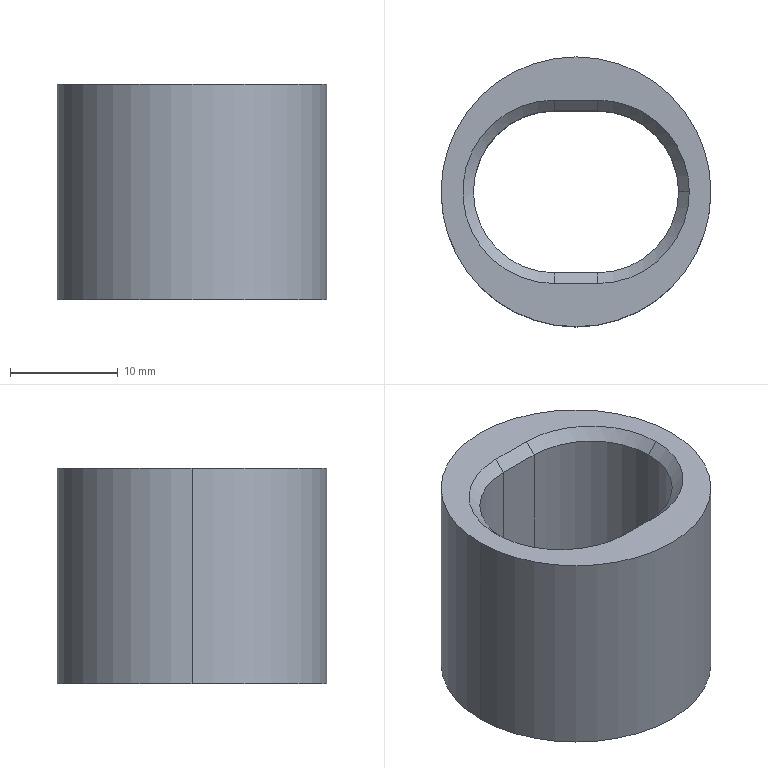Part | SolidWorks | features Chamfer 1, Extrusion 1 | 1 solid | 14 faces | box 25 x 25 x 20 mm | volume 5055 mm3 | plane 6 | cylinder 5 | cone 3 | commonest cylinder face diameters 15 x3 25 x2
STEP:
#1=CARTESIAN_POINT('',(9.5,0.,19.));
#2=VERTEX_POINT('',#1);
#3=CARTESIAN_POINT('',(2.,7.5,19.));
#4=VERTEX_POINT('',#3);
#5=CARTESIAN_POINT('',(2.,0.,19.));
#6=DIRECTION('',(0.,0.,1.));
#7=DIRECTION('',(1.,0.,0.));
#8=AXIS2_PLACEMENT_3D('',#5,#6,#7);
#9=CIRCLE('',#8,7.5);
#10=EDGE_CURVE('',#2,#4,#9,.T.);
#11=ORIENTED_EDGE('',*,*,#10,.F.);
#12=CARTESIAN_POINT('',(10.5,0.,20.));
#13=VERTEX_POINT('',#12);
#14=CARTESIAN_POINT('',(9.5,0.,19.));
#15=DIRECTION('',(0.7071,0.,0.7071));
#16=VECTOR('',#15,1000.);
#17=LINE('',#14,#16);
#18=EDGE_CURVE('',#2,#13,#17,.T.);
#19=ORIENTED_EDGE('',*,*,#18,.T.);
#20=CARTESIAN_POINT('',(2.,8.5,20.));
#21=VERTEX_POINT('',#20);
#22=CARTESIAN_POINT('',(2.,0.,20.));
#23=DIRECTION('',(0.,0.,-1.));
#24=DIRECTION('',(1.,0.,0.));
#25=AXIS2_PLACEMENT_3D('',#22,#23,#24);
#26=CIRCLE('',#25,8.5);
#27=EDGE_CURVE('',#21,#13,#26,.T.);
#28=ORIENTED_EDGE('',*,*,#27,.F.);
#29=CARTESIAN_POINT('',(2.,8.5,20.));
#30=DIRECTION('',(0.,-0.7071,-0.7071));
#31=VECTOR('',#30,1000.);
#32=LINE('',#29,#31);
#33=EDGE_CURVE('',#21,#4,#32,.T.);
#34=ORIENTED_EDGE('',*,*,#33,.T.);
#35=EDGE_LOOP('',(#11,#19,#28,#34));
#36=FACE_OUTER_BOUND('',#35,.T.);
#37=CARTESIAN_POINT('',(2.,0.,19.));
#38=DIRECTION('',(0.,0.,1.));
#39=DIRECTION('',(1.,0.,0.));
#40=AXIS2_PLACEMENT_3D('',#37,#38,#39);
#41=CONICAL_SURFACE('',#40,7.5,0.7854);
#42=ADVANCED_FACE('',(#36),#41,.F.);
#43=CARTESIAN_POINT('',(-2.,7.5,19.));
#44=VERTEX_POINT('',#43);
#45=CARTESIAN_POINT('',(-9.5,0.,19.));
#46=VERTEX_POINT('',#45);
#47=CARTESIAN_POINT('',(-2.,0.,19.));
#48=DIRECTION('',(0.,0.,1.));
#49=DIRECTION('',(1.,0.,0.));
#50=AXIS2_PLACEMENT_3D('',#47,#48,#49);
#51=CIRCLE('',#50,7.5);
#52=EDGE_CURVE('',#44,#46,#51,.T.);
#53=ORIENTED_EDGE('',*,*,#52,.T.);
#54=CARTESIAN_POINT('',(-9.5,0.,0.));
#55=VERTEX_POINT('',#54);
#56=CARTESIAN_POINT('',(-9.5,0.,20.));
#57=DIRECTION('',(0.,0.,-1.));
#58=VECTOR('',#57,1000.);
#59=LINE('',#56,#58);
#60=EDGE_CURVE('',#46,#55,#59,.T.);
#61=ORIENTED_EDGE('',*,*,#60,.T.);
#62=CARTESIAN_POINT('',(-2.,7.5,0.));
#63=VERTEX_POINT('',#62);
#64=CARTESIAN_POINT('',(-2.,0.,0.));
#65=DIRECTION('',(0.,0.,1.));
#66=DIRECTION('',(1.,0.,0.));
#67=AXIS2_PLACEMENT_3D('',#64,#65,#66);
#68=CIRCLE('',#67,7.5);
#69=EDGE_CURVE('',#63,#55,#68,.T.);
#70=ORIENTED_EDGE('',*,*,#69,.F.);
#71=CARTESIAN_POINT('',(-2.,7.5,20.));
#72=DIRECTION('',(0.,0.,-1.));
#73=VECTOR('',#72,1000.);
#74=LINE('',#71,#73);
#75=EDGE_CURVE('',#44,#63,#74,.T.);
#76=ORIENTED_EDGE('',*,*,#75,.F.);
#77=EDGE_LOOP('',(#53,#61,#70,#76));
#78=FACE_OUTER_BOUND('',#77,.T.);
#79=CARTESIAN_POINT('',(-2.,0.,20.));
#80=DIRECTION('',(0.,0.,-1.));
#81=DIRECTION('',(-1.,0.,0.));
#82=AXIS2_PLACEMENT_3D('',#79,#80,#81);
#83=CYLINDRICAL_SURFACE('',#82,7.5);
#84=ADVANCED_FACE('',(#78),#83,.F.);
#85=CARTESIAN_POINT('',(12.5,0.,20.));
#86=VERTEX_POINT('',#85);
#87=CARTESIAN_POINT('',(-12.5,0.,20.));
#88=VERTEX_POINT('',#87);
#89=CARTESIAN_POINT('',(0.,0.,20.));
#90=DIRECTION('',(0.,0.,1.));
#91=DIRECTION('',(1.,0.,0.));
#92=AXIS2_PLACEMENT_3D('',#89,#90,#91);
#93=CIRCLE('',#92,12.5);
#94=EDGE_CURVE('',#86,#88,#93,.T.);
#95=ORIENTED_EDGE('',*,*,#94,.F.);
#96=CARTESIAN_POINT('',(12.5,0.,0.));
#97=VERTEX_POINT('',#96);
#98=CARTESIAN_POINT('',(12.5,0.,20.));
#99=DIRECTION('',(0.,0.,-1.));
#100=VECTOR('',#99,1000.);
#101=LINE('',#98,#100);
#102=EDGE_CURVE('',#86,#97,#101,.T.);
#103=ORIENTED_EDGE('',*,*,#102,.T.);
#104=CARTESIAN_POINT('',(-12.5,0.,0.));
#105=VERTEX_POINT('',#104);
#106=CARTESIAN_POINT('',(0.,0.,0.));
#107=DIRECTION('',(0.,0.,1.));
#108=DIRECTION('',(1.,0.,0.));
#109=AXIS2_PLACEMENT_3D('',#106,#107,#108);
#110=CIRCLE('',#109,12.5);
#111=EDGE_CURVE('',#97,#105,#110,.T.);
#112=ORIENTED_EDGE('',*,*,#111,.T.);
#113=CARTESIAN_POINT('',(-12.5,0.,20.));
#114=DIRECTION('',(0.,0.,-1.));
#115=VECTOR('',#114,1000.);
#116=LINE('',#113,#115);
#117=EDGE_CURVE('',#88,#105,#116,.T.);
#118=ORIENTED_EDGE('',*,*,#117,.F.);
#119=EDGE_LOOP('',(#95,#103,#112,#118));
#120=FACE_OUTER_BOUND('',#119,.T.);
#121=CARTESIAN_POINT('',(0.,0.,20.));
#122=DIRECTION('',(0.,0.,-1.));
#123=DIRECTION('',(-1.,0.,0.));
#124=AXIS2_PLACEMENT_3D('',#121,#122,#123);
#125=CYLINDRICAL_SURFACE('',#124,12.5);
#126=ADVANCED_FACE('',(#120),#125,.T.);
#127=ORIENTED_EDGE('',*,*,#27,.T.);
#128=CARTESIAN_POINT('',(2.,-8.5,20.));
#129=VERTEX_POINT('',#128);
#130=CARTESIAN_POINT('',(2.,0.,20.));
#131=DIRECTION('',(0.,0.,-1.));
#132=DIRECTION('',(1.,0.,0.));
#133=AXIS2_PLACEMENT_3D('',#130,#131,#132);
#134=CIRCLE('',#133,8.5);
#135=EDGE_CURVE('',#13,#129,#134,.T.);
#136=ORIENTED_EDGE('',*,*,#135,.T.);
#137=CARTESIAN_POINT('',(-2.,-8.5,20.));
#138=VERTEX_POINT('',#137);
#139=CARTESIAN_POINT('',(0.,-8.5,20.));
#140=DIRECTION('',(-1.,0.,0.));
#141=VECTOR('',#140,1000.);
#142=LINE('',#139,#141);
#143=EDGE_CURVE('',#129,#138,#142,.T.);
#144=ORIENTED_EDGE('',*,*,#143,.T.);
#145=CARTESIAN_POINT('',(-2.,8.5,20.));
#146=VERTEX_POINT('',#145);
#147=CARTESIAN_POINT('',(-2.,0.,20.));
#148=DIRECTION('',(0.,0.,-1.));
#149=DIRECTION('',(1.,0.,0.));
#150=AXIS2_PLACEMENT_3D('',#147,#148,#149);
#151=CIRCLE('',#150,8.5);
#152=EDGE_CURVE('',#138,#146,#151,.T.);
#153=ORIENTED_EDGE('',*,*,#152,.T.);
#154=CARTESIAN_POINT('',(0.,8.5,20.));
#155=DIRECTION('',(1.,0.,0.));
#156=VECTOR('',#155,1000.);
#157=LINE('',#154,#156);
#158=EDGE_CURVE('',#146,#21,#157,.T.);
#159=ORIENTED_EDGE('',*,*,#158,.T.);
#160=EDGE_LOOP('',(#127,#136,#144,#153,#159));
#161=FACE_BOUND('',#160,.T.);
#162=CARTESIAN_POINT('',(0.,0.,20.));
#163=DIRECTION('',(0.,0.,1.));
#164=DIRECTION('',(1.,0.,0.));
#165=AXIS2_PLACEMENT_3D('',#162,#163,#164);
#166=CIRCLE('',#165,12.5);
#167=EDGE_CURVE('',#88,#86,#166,.T.);
#168=ORIENTED_EDGE('',*,*,#167,.T.);
#169=ORIENTED_EDGE('',*,*,#94,.T.);
#170=EDGE_LOOP('',(#168,#169));
#171=FACE_OUTER_BOUND('',#170,.T.);
#172=CARTESIAN_POINT('',(0.,0.,20.));
#173=DIRECTION('',(0.,0.,1.));
#174=DIRECTION('',(1.,0.,0.));
#175=AXIS2_PLACEMENT_3D('',#172,#173,#174);
#176=PLANE('',#175);
#177=ADVANCED_FACE('',(#161,#171),#176,.T.);
#178=CARTESIAN_POINT('',(0.,0.,0.));
#179=DIRECTION('',(0.,0.,1.));
#180=DIRECTION('',(1.,0.,0.));
#181=AXIS2_PLACEMENT_3D('',#178,#179,#180);
#182=CIRCLE('',#181,12.5);
#183=EDGE_CURVE('',#105,#97,#182,.T.);
#184=ORIENTED_EDGE('',*,*,#183,.F.);
#185=ORIENTED_EDGE('',*,*,#111,.F.);
#186=EDGE_LOOP('',(#184,#185));
#187=FACE_OUTER_BOUND('',#186,.T.);
#188=ORIENTED_EDGE('',*,*,#69,.T.);
#189=CARTESIAN_POINT('',(-2.,-7.5,0.));
#190=VERTEX_POINT('',#189);
#191=CARTESIAN_POINT('',(-2.,0.,0.));
#192=DIRECTION('',(0.,0.,1.));
#193=DIRECTION('',(1.,0.,0.));
#194=AXIS2_PLACEMENT_3D('',#191,#192,#193);
#195=CIRCLE('',#194,7.5);
#196=EDGE_CURVE('',#55,#190,#195,.T.);
#197=ORIENTED_EDGE('',*,*,#196,.T.);
#198=CARTESIAN_POINT('',(2.,-7.5,0.));
#199=VERTEX_POINT('',#198);
#200=CARTESIAN_POINT('',(-2.,-7.5,0.));
#201=DIRECTION('',(1.,0.,0.));
#202=VECTOR('',#201,1000.);
#203=LINE('',#200,#202);
#204=EDGE_CURVE('',#190,#199,#203,.T.);
#205=ORIENTED_EDGE('',*,*,#204,.T.);
#206=CARTESIAN_POINT('',(2.,7.5,0.));
#207=VERTEX_POINT('',#206);
#208=CARTESIAN_POINT('',(2.,0.,0.));
#209=DIRECTION('',(0.,0.,1.));
#210=DIRECTION('',(1.,0.,0.));
#211=AXIS2_PLACEMENT_3D('',#208,#209,#210);
#212=CIRCLE('',#211,7.5);
#213=EDGE_CURVE('',#199,#207,#212,.T.);
#214=ORIENTED_EDGE('',*,*,#213,.T.);
#215=CARTESIAN_POINT('',(-2.,7.5,0.));
#216=DIRECTION('',(-1.,0.,0.));
#217=VECTOR('',#216,1000.);
#218=LINE('',#215,#217);
#219=EDGE_CURVE('',#207,#63,#218,.T.);
#220=ORIENTED_EDGE('',*,*,#219,.T.);
#221=EDGE_LOOP('',(#188,#197,#205,#214,#220));
#222=FACE_BOUND('',#221,.T.);
#223=CARTESIAN_POINT('',(0.,0.,0.));
#224=DIRECTION('',(0.,0.,1.));
#225=DIRECTION('',(1.,0.,0.));
#226=AXIS2_PLACEMENT_3D('',#223,#224,#225);
#227=PLANE('',#226);
#228=ADVANCED_FACE('',(#187,#222),#227,.F.);
#229=ORIENTED_EDGE('',*,*,#102,.F.);
#230=ORIENTED_EDGE('',*,*,#167,.F.);
#231=ORIENTED_EDGE('',*,*,#117,.T.);
#232=ORIENTED_EDGE('',*,*,#183,.T.);
#233=EDGE_LOOP('',(#229,#230,#231,#232));
#234=FACE_OUTER_BOUND('',#233,.T.);
#235=CARTESIAN_POINT('',(0.,0.,20.));
#236=DIRECTION('',(0.,0.,-1.));
#237=DIRECTION('',(-1.,0.,0.));
#238=AXIS2_PLACEMENT_3D('',#235,#236,#237);
#239=CYLINDRICAL_SURFACE('',#238,12.5);
#240=ADVANCED_FACE('',(#234),#239,.T.);
#241=ORIENTED_EDGE('',*,*,#60,.F.);
#242=CARTESIAN_POINT('',(-2.,-7.5,19.));
#243=VERTEX_POINT('',#242);
#244=CARTESIAN_POINT('',(-2.,0.,19.));
#245=DIRECTION('',(0.,0.,1.));
#246=DIRECTION('',(1.,0.,0.));
#247=AXIS2_PLACEMENT_3D('',#244,#245,#246);
#248=CIRCLE('',#247,7.5);
#249=EDGE_CURVE('',#46,#243,#248,.T.);
#250=ORIENTED_EDGE('',*,*,#249,.T.);
#251=CARTESIAN_POINT('',(-2.,-7.5,20.));
#252=DIRECTION('',(0.,0.,-1.));
#253=VECTOR('',#252,1000.);
#254=LINE('',#251,#253);
#255=EDGE_CURVE('',#243,#190,#254,.T.);
#256=ORIENTED_EDGE('',*,*,#255,.T.);
#257=ORIENTED_EDGE('',*,*,#196,.F.);
#258=EDGE_LOOP('',(#241,#250,#256,#257));
#259=FACE_OUTER_BOUND('',#258,.T.);
#260=CARTESIAN_POINT('',(-2.,0.,20.));
#261=DIRECTION('',(0.,0.,-1.));
#262=DIRECTION('',(-1.,0.,0.));
#263=AXIS2_PLACEMENT_3D('',#260,#261,#262);
#264=CYLINDRICAL_SURFACE('',#263,7.5);
#265=ADVANCED_FACE('',(#259),#264,.F.);
#266=ORIENTED_EDGE('',*,*,#255,.F.);
#267=CARTESIAN_POINT('',(2.,-7.5,19.));
#268=VERTEX_POINT('',#267);
#269=CARTESIAN_POINT('',(-2.,-7.5,19.));
#270=DIRECTION('',(1.,0.,0.));
#271=VECTOR('',#270,1000.);
#272=LINE('',#269,#271);
#273=EDGE_CURVE('',#243,#268,#272,.T.);
#274=ORIENTED_EDGE('',*,*,#273,.T.);
#275=CARTESIAN_POINT('',(2.,-7.5,20.));
#276=DIRECTION('',(0.,0.,-1.));
#277=VECTOR('',#276,1000.);
#278=LINE('',#275,#277);
#279=EDGE_CURVE('',#268,#199,#278,.T.);
#280=ORIENTED_EDGE('',*,*,#279,.T.);
#281=ORIENTED_EDGE('',*,*,#204,.F.);
#282=EDGE_LOOP('',(#266,#274,#280,#281));
#283=FACE_OUTER_BOUND('',#282,.T.);
#284=CARTESIAN_POINT('',(-2.,-7.5,20.));
#285=DIRECTION('',(0.,1.,0.));
#286=DIRECTION('',(0.,0.,1.));
#287=AXIS2_PLACEMENT_3D('',#284,#285,#286);
#288=PLANE('',#287);
#289=ADVANCED_FACE('',(#283),#288,.T.);
#290=ORIENTED_EDGE('',*,*,#279,.F.);
#291=CARTESIAN_POINT('',(2.,0.,19.));
#292=DIRECTION('',(0.,0.,1.));
#293=DIRECTION('',(1.,0.,0.));
#294=AXIS2_PLACEMENT_3D('',#291,#292,#293);
#295=CIRCLE('',#294,7.5);
#296=EDGE_CURVE('',#268,#2,#295,.T.);
#297=ORIENTED_EDGE('',*,*,#296,.T.);
#298=ORIENTED_EDGE('',*,*,#10,.T.);
#299=CARTESIAN_POINT('',(2.,7.5,20.));
#300=DIRECTION('',(0.,0.,-1.));
#301=VECTOR('',#300,1000.);
#302=LINE('',#299,#301);
#303=EDGE_CURVE('',#4,#207,#302,.T.);
#304=ORIENTED_EDGE('',*,*,#303,.T.);
#305=ORIENTED_EDGE('',*,*,#213,.F.);
#306=EDGE_LOOP('',(#290,#297,#298,#304,#305));
#307=FACE_OUTER_BOUND('',#306,.T.);
#308=CARTESIAN_POINT('',(2.,0.,20.));
#309=DIRECTION('',(0.,0.,-1.));
#310=DIRECTION('',(-1.,0.,0.));
#311=AXIS2_PLACEMENT_3D('',#308,#309,#310);
#312=CYLINDRICAL_SURFACE('',#311,7.5);
#313=ADVANCED_FACE('',(#307),#312,.F.);
#314=ORIENTED_EDGE('',*,*,#303,.F.);
#315=CARTESIAN_POINT('',(-2.,7.5,19.));
#316=DIRECTION('',(-1.,0.,0.));
#317=VECTOR('',#316,1000.);
#318=LINE('',#315,#317);
#319=EDGE_CURVE('',#4,#44,#318,.T.);
#320=ORIENTED_EDGE('',*,*,#319,.T.);
#321=ORIENTED_EDGE('',*,*,#75,.T.);
#322=ORIENTED_EDGE('',*,*,#219,.F.);
#323=EDGE_LOOP('',(#314,#320,#321,#322));
#324=FACE_OUTER_BOUND('',#323,.T.);
#325=CARTESIAN_POINT('',(-2.,7.5,20.));
#326=DIRECTION('',(0.,-1.,0.));
#327=DIRECTION('',(0.,0.,-1.));
#328=AXIS2_PLACEMENT_3D('',#325,#326,#327);
#329=PLANE('',#328);
#330=ADVANCED_FACE('',(#324),#329,.T.);
#331=ORIENTED_EDGE('',*,*,#33,.F.);
#332=ORIENTED_EDGE('',*,*,#158,.F.);
#333=CARTESIAN_POINT('',(-2.,7.5,19.));
#334=DIRECTION('',(0.,0.7071,0.7071));
#335=VECTOR('',#334,1000.);
#336=LINE('',#333,#335);
#337=EDGE_CURVE('',#44,#146,#336,.T.);
#338=ORIENTED_EDGE('',*,*,#337,.F.);
#339=ORIENTED_EDGE('',*,*,#319,.F.);
#340=EDGE_LOOP('',(#331,#332,#338,#339));
#341=FACE_OUTER_BOUND('',#340,.T.);
#342=CARTESIAN_POINT('',(-2.,7.5,19.));
#343=DIRECTION('',(0.,0.7071,-0.7071));
#344=DIRECTION('',(-1.,0.,0.));
#345=AXIS2_PLACEMENT_3D('',#342,#343,#344);
#346=PLANE('',#345);
#347=ADVANCED_FACE('',(#341),#346,.F.);
#348=ORIENTED_EDGE('',*,*,#337,.T.);
#349=ORIENTED_EDGE('',*,*,#152,.F.);
#350=CARTESIAN_POINT('',(-2.,-7.5,19.));
#351=DIRECTION('',(0.,-0.7071,0.7071));
#352=VECTOR('',#351,1000.);
#353=LINE('',#350,#352);
#354=EDGE_CURVE('',#243,#138,#353,.T.);
#355=ORIENTED_EDGE('',*,*,#354,.F.);
#356=ORIENTED_EDGE('',*,*,#249,.F.);
#357=ORIENTED_EDGE('',*,*,#52,.F.);
#358=EDGE_LOOP('',(#348,#349,#355,#356,#357));
#359=FACE_OUTER_BOUND('',#358,.T.);
#360=CARTESIAN_POINT('',(-2.,0.,19.));
#361=DIRECTION('',(0.,0.,1.));
#362=DIRECTION('',(1.,0.,0.));
#363=AXIS2_PLACEMENT_3D('',#360,#361,#362);
#364=CONICAL_SURFACE('',#363,7.5,0.7854);
#365=ADVANCED_FACE('',(#359),#364,.F.);
#366=ORIENTED_EDGE('',*,*,#18,.F.);
#367=ORIENTED_EDGE('',*,*,#296,.F.);
#368=CARTESIAN_POINT('',(2.,-8.5,20.));
#369=DIRECTION('',(0.,0.7071,-0.7071));
#370=VECTOR('',#369,1000.);
#371=LINE('',#368,#370);
#372=EDGE_CURVE('',#129,#268,#371,.T.);
#373=ORIENTED_EDGE('',*,*,#372,.F.);
#374=ORIENTED_EDGE('',*,*,#135,.F.);
#375=EDGE_LOOP('',(#366,#367,#373,#374));
#376=FACE_OUTER_BOUND('',#375,.T.);
#377=CARTESIAN_POINT('',(2.,0.,19.));
#378=DIRECTION('',(0.,0.,1.));
#379=DIRECTION('',(1.,0.,0.));
#380=AXIS2_PLACEMENT_3D('',#377,#378,#379);
#381=CONICAL_SURFACE('',#380,7.5,0.7854);
#382=ADVANCED_FACE('',(#376),#381,.F.);
#383=ORIENTED_EDGE('',*,*,#354,.T.);
#384=ORIENTED_EDGE('',*,*,#143,.F.);
#385=ORIENTED_EDGE('',*,*,#372,.T.);
#386=ORIENTED_EDGE('',*,*,#273,.F.);
#387=EDGE_LOOP('',(#383,#384,#385,#386));
#388=FACE_OUTER_BOUND('',#387,.T.);
#389=CARTESIAN_POINT('',(-2.,-7.5,19.));
#390=DIRECTION('',(0.,-0.7071,-0.7071));
#391=DIRECTION('',(1.,0.,0.));
#392=AXIS2_PLACEMENT_3D('',#389,#390,#391);
#393=PLANE('',#392);
#394=ADVANCED_FACE('',(#388),#393,.F.);
#395=CLOSED_SHELL('',(#42,#84,#126,#177,#228,#240,#265,#289,#313,#330,#347,#365,#382,#394));
#396=MANIFOLD_SOLID_BREP('',#395);
#397=CARTESIAN_POINT('',(0.,0.,0.));
#398=DIRECTION('',(0.,0.,1.));
#399=DIRECTION('',(1.,0.,0.));
#400=AXIS2_PLACEMENT_3D('',#397,#398,#399);
#401=(LENGTH_UNIT()NAMED_UNIT(*)SI_UNIT(.MILLI.,.METRE.));
#402=UNCERTAINTY_MEASURE_WITH_UNIT(LENGTH_MEASURE(0.00001),#401,'','');
#403=(NAMED_UNIT(*)PLANE_ANGLE_UNIT()SI_UNIT($,.RADIAN.));
#404=(NAMED_UNIT(*)SI_UNIT($,.STERADIAN.)SOLID_ANGLE_UNIT());
#405=(GEOMETRIC_REPRESENTATION_CONTEXT(3)GLOBAL_UNCERTAINTY_ASSIGNED_CONTEXT((#402))GLOBAL_UNIT_ASSIGNED_CONTEXT((#401,#403,#404))REPRESENTATION_CONTEXT('',''));
#406=ADVANCED_BREP_SHAPE_REPRESENTATION('',(#396,#400),#405);